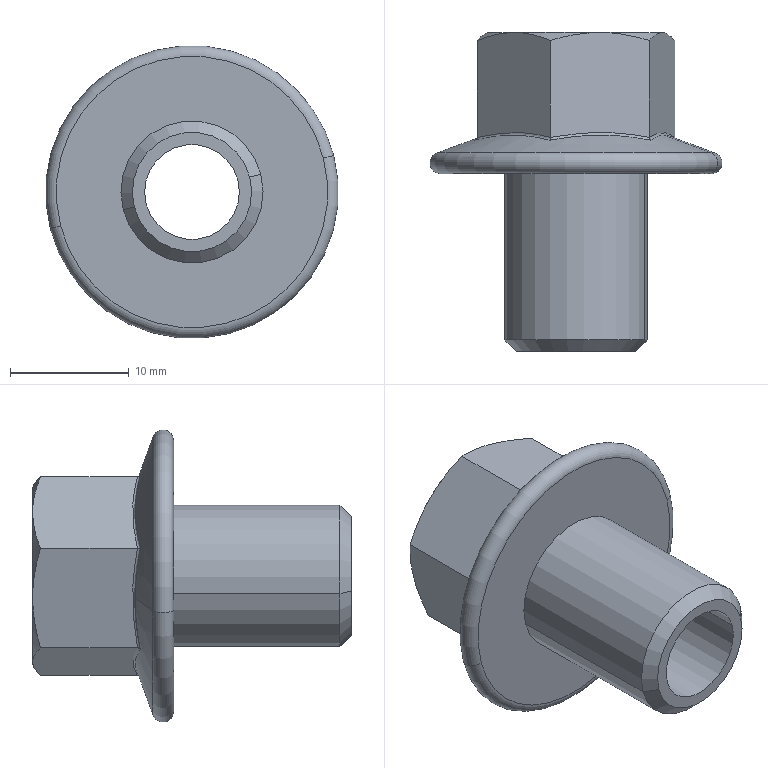Part | STEP file | Input 139 | 1 solid | 31 faces | box 24.7 x 26.9 x 24.7 mm | volume 3275 mm3 | cone 10 | plane 9 | spline 6 | cylinder 4 | torus 2 | commonest cylinder face diameters 8 x2 12 x2